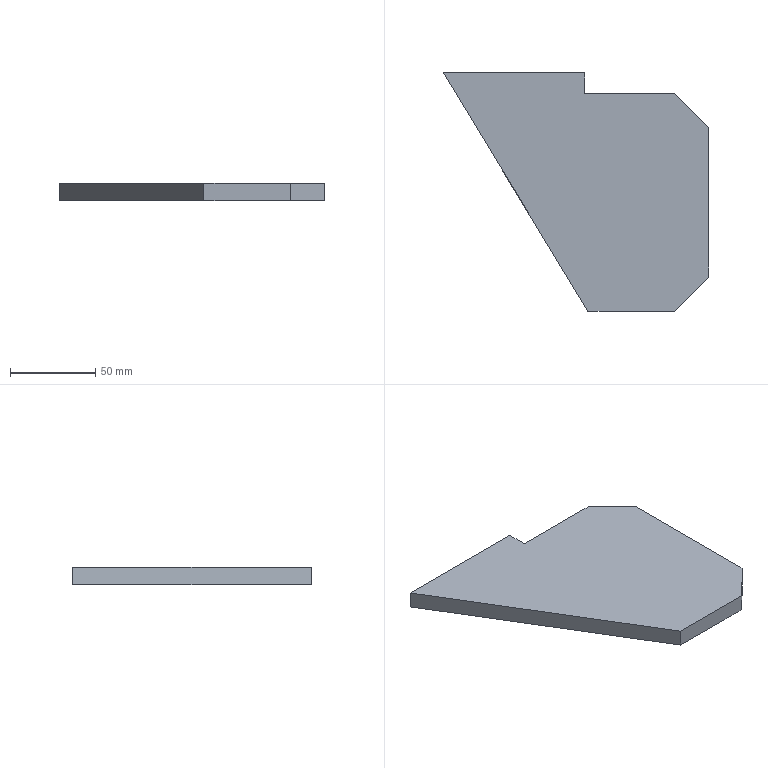Part | STEP file | 07 Rib plate | 1 solid | 10 faces | box 156 x 140 x 10 mm | volume 146140 mm3 | plane 10
STEP:
#1=CARTESIAN_POINT('',(0.,0.,0.));
#2=DIRECTION('',(0.,0.,1.));
#3=DIRECTION('',(1.,0.,0.));
#4=AXIS2_PLACEMENT_3D('',#1,#2,#3);
#5=CARTESIAN_POINT('',(0.,0.,0.));
#6=VERTEX_POINT('',#5);
#7=CARTESIAN_POINT('',(85.,-140.,0.));
#8=VERTEX_POINT('',#7);
#9=CARTESIAN_POINT('',(0.,0.,0.));
#10=DIRECTION('',(0.519,-0.8548,0.));
#11=VECTOR('',#10,1.);
#12=LINE('',#9,#11);
#13=CARTESIAN_POINT('',(0.,0.,10.));
#14=DIRECTION('',(0.8548,0.519,0.));
#15=DIRECTION('',(-0.519,0.8548,0.));
#16=AXIS2_PLACEMENT_3D('',#13,#14,#15);
#17=PLANE('',#16);
#18=CARTESIAN_POINT('',(0.,-10.));
#19=DIRECTION('',(-1.,0.));
#20=VECTOR('',#19,1.);
#21=LINE('',#18,#20);
#22=(GEOMETRIC_REPRESENTATION_CONTEXT(2)PARAMETRIC_REPRESENTATION_CONTEXT()REPRESENTATION_CONTEXT('',''));
#23=DEFINITIONAL_REPRESENTATION('',(#21),#22);
#24=PCURVE('',#17,#23);
#25=CARTESIAN_POINT('',(0.,0.,0.));
#26=DIRECTION('',(0.,0.,-1.));
#27=DIRECTION('',(-1.,0.,0.));
#28=AXIS2_PLACEMENT_3D('',#25,#26,#27);
#29=PLANE('',#28);
#30=CARTESIAN_POINT('',(0.,0.));
#31=DIRECTION('',(-0.519,-0.8548));
#32=VECTOR('',#31,1.);
#33=LINE('',#30,#32);
#34=(GEOMETRIC_REPRESENTATION_CONTEXT(2)PARAMETRIC_REPRESENTATION_CONTEXT()REPRESENTATION_CONTEXT('',''));
#35=DEFINITIONAL_REPRESENTATION('',(#33),#34);
#36=PCURVE('',#29,#35);
#37=SURFACE_CURVE('',#12,(#24,#36),.PCURVE_S1.);
#38=EDGE_CURVE('',#6,#8,#37,.T.);
#39=ORIENTED_EDGE('',*,*,#38,.T.);
#40=CARTESIAN_POINT('',(85.,-140.,10.));
#41=VERTEX_POINT('',#40);
#42=CARTESIAN_POINT('',(85.,-140.,10.));
#43=DIRECTION('',(0.,0.,-1.));
#44=VECTOR('',#43,1.);
#45=LINE('',#42,#44);
#46=CARTESIAN_POINT('',(-163.783,0.));
#47=DIRECTION('',(0.,-1.));
#48=VECTOR('',#47,1.);
#49=LINE('',#46,#48);
#50=(GEOMETRIC_REPRESENTATION_CONTEXT(2)PARAMETRIC_REPRESENTATION_CONTEXT()REPRESENTATION_CONTEXT('',''));
#51=DEFINITIONAL_REPRESENTATION('',(#49),#50);
#52=PCURVE('',#17,#51);
#53=CARTESIAN_POINT('',(85.,-140.,10.));
#54=DIRECTION('',(0.,1.,0.));
#55=DIRECTION('',(0.,0.,1.));
#56=AXIS2_PLACEMENT_3D('',#53,#54,#55);
#57=PLANE('',#56);
#58=CARTESIAN_POINT('',(0.,0.));
#59=DIRECTION('',(-1.,0.));
#60=VECTOR('',#59,1.);
#61=LINE('',#58,#60);
#62=(GEOMETRIC_REPRESENTATION_CONTEXT(2)PARAMETRIC_REPRESENTATION_CONTEXT()REPRESENTATION_CONTEXT('',''));
#63=DEFINITIONAL_REPRESENTATION('',(#61),#62);
#64=PCURVE('',#57,#63);
#65=SURFACE_CURVE('',#45,(#52,#64),.PCURVE_S1.);
#66=EDGE_CURVE('',#41,#8,#65,.T.);
#67=ORIENTED_EDGE('',*,*,#66,.F.);
#68=CARTESIAN_POINT('',(0.,0.,10.));
#69=VERTEX_POINT('',#68);
#70=CARTESIAN_POINT('',(0.,0.,10.));
#71=DIRECTION('',(0.519,-0.8548,0.));
#72=VECTOR('',#71,1.);
#73=LINE('',#70,#72);
#74=CARTESIAN_POINT('',(0.,0.));
#75=DIRECTION('',(-1.,0.));
#76=VECTOR('',#75,1.);
#77=LINE('',#74,#76);
#78=(GEOMETRIC_REPRESENTATION_CONTEXT(2)PARAMETRIC_REPRESENTATION_CONTEXT()REPRESENTATION_CONTEXT('',''));
#79=DEFINITIONAL_REPRESENTATION('',(#77),#78);
#80=PCURVE('',#17,#79);
#81=CARTESIAN_POINT('',(0.,0.,10.));
#82=DIRECTION('',(0.,0.,-1.));
#83=DIRECTION('',(-1.,0.,0.));
#84=AXIS2_PLACEMENT_3D('',#81,#82,#83);
#85=PLANE('',#84);
#86=CARTESIAN_POINT('',(0.,0.));
#87=DIRECTION('',(-0.519,-0.8548));
#88=VECTOR('',#87,1.);
#89=LINE('',#86,#88);
#90=(GEOMETRIC_REPRESENTATION_CONTEXT(2)PARAMETRIC_REPRESENTATION_CONTEXT()REPRESENTATION_CONTEXT('',''));
#91=DEFINITIONAL_REPRESENTATION('',(#89),#90);
#92=PCURVE('',#85,#91);
#93=SURFACE_CURVE('',#73,(#80,#92),.PCURVE_S1.);
#94=EDGE_CURVE('',#69,#41,#93,.T.);
#95=ORIENTED_EDGE('',*,*,#94,.F.);
#96=CARTESIAN_POINT('',(0.,0.,10.));
#97=DIRECTION('',(0.,0.,-1.));
#98=VECTOR('',#97,1.);
#99=LINE('',#96,#98);
#100=CARTESIAN_POINT('',(0.,0.));
#101=DIRECTION('',(0.,-1.));
#102=VECTOR('',#101,1.);
#103=LINE('',#100,#102);
#104=(GEOMETRIC_REPRESENTATION_CONTEXT(2)PARAMETRIC_REPRESENTATION_CONTEXT()REPRESENTATION_CONTEXT('',''));
#105=DEFINITIONAL_REPRESENTATION('',(#103),#104);
#106=PCURVE('',#17,#105);
#107=CARTESIAN_POINT('',(0.,0.,10.));
#108=DIRECTION('',(0.,-1.,0.));
#109=DIRECTION('',(0.,0.,-1.));
#110=AXIS2_PLACEMENT_3D('',#107,#108,#109);
#111=PLANE('',#110);
#112=CARTESIAN_POINT('',(0.,0.));
#113=DIRECTION('',(1.,0.));
#114=VECTOR('',#113,1.);
#115=LINE('',#112,#114);
#116=(GEOMETRIC_REPRESENTATION_CONTEXT(2)PARAMETRIC_REPRESENTATION_CONTEXT()REPRESENTATION_CONTEXT('',''));
#117=DEFINITIONAL_REPRESENTATION('',(#115),#116);
#118=PCURVE('',#111,#117);
#119=SURFACE_CURVE('',#99,(#106,#118),.PCURVE_S1.);
#120=EDGE_CURVE('',#69,#6,#119,.T.);
#121=ORIENTED_EDGE('',*,*,#120,.T.);
#122=EDGE_LOOP('',(#39,#67,#95,#121));
#123=FACE_BOUND('',#122,.T.);
#124=ADVANCED_FACE('',(#123),#17,.F.);
#125=CARTESIAN_POINT('',(136.,-140.,0.));
#126=VERTEX_POINT('',#125);
#127=CARTESIAN_POINT('',(85.,-140.,0.));
#128=DIRECTION('',(1.,0.,0.));
#129=VECTOR('',#128,1.);
#130=LINE('',#127,#129);
#131=CARTESIAN_POINT('',(-10.,0.));
#132=DIRECTION('',(0.,1.));
#133=VECTOR('',#132,1.);
#134=LINE('',#131,#133);
#135=(GEOMETRIC_REPRESENTATION_CONTEXT(2)PARAMETRIC_REPRESENTATION_CONTEXT()REPRESENTATION_CONTEXT('',''));
#136=DEFINITIONAL_REPRESENTATION('',(#134),#135);
#137=PCURVE('',#57,#136);
#138=CARTESIAN_POINT('',(-85.,-140.));
#139=DIRECTION('',(-1.,0.));
#140=VECTOR('',#139,1.);
#141=LINE('',#138,#140);
#142=(GEOMETRIC_REPRESENTATION_CONTEXT(2)PARAMETRIC_REPRESENTATION_CONTEXT()REPRESENTATION_CONTEXT('',''));
#143=DEFINITIONAL_REPRESENTATION('',(#141),#142);
#144=PCURVE('',#29,#143);
#145=SURFACE_CURVE('',#130,(#137,#144),.PCURVE_S1.);
#146=EDGE_CURVE('',#8,#126,#145,.T.);
#147=ORIENTED_EDGE('',*,*,#146,.T.);
#148=CARTESIAN_POINT('',(136.,-140.,10.));
#149=VERTEX_POINT('',#148);
#150=CARTESIAN_POINT('',(136.,-140.,10.));
#151=DIRECTION('',(0.,0.,-1.));
#152=VECTOR('',#151,1.);
#153=LINE('',#150,#152);
#154=CARTESIAN_POINT('',(0.,51.));
#155=DIRECTION('',(-1.,0.));
#156=VECTOR('',#155,1.);
#157=LINE('',#154,#156);
#158=(GEOMETRIC_REPRESENTATION_CONTEXT(2)PARAMETRIC_REPRESENTATION_CONTEXT()REPRESENTATION_CONTEXT('',''));
#159=DEFINITIONAL_REPRESENTATION('',(#157),#158);
#160=PCURVE('',#57,#159);
#161=CARTESIAN_POINT('',(156.,-120.,10.));
#162=DIRECTION('',(-0.7071,0.7071,0.));
#163=DIRECTION('',(-0.7071,-0.7071,0.));
#164=AXIS2_PLACEMENT_3D('',#161,#162,#163);
#165=PLANE('',#164);
#166=CARTESIAN_POINT('',(28.284,0.));
#167=DIRECTION('',(0.,-1.));
#168=VECTOR('',#167,1.);
#169=LINE('',#166,#168);
#170=(GEOMETRIC_REPRESENTATION_CONTEXT(2)PARAMETRIC_REPRESENTATION_CONTEXT()REPRESENTATION_CONTEXT('',''));
#171=DEFINITIONAL_REPRESENTATION('',(#169),#170);
#172=PCURVE('',#165,#171);
#173=SURFACE_CURVE('',#153,(#160,#172),.PCURVE_S1.);
#174=EDGE_CURVE('',#149,#126,#173,.T.);
#175=ORIENTED_EDGE('',*,*,#174,.F.);
#176=CARTESIAN_POINT('',(85.,-140.,10.));
#177=DIRECTION('',(1.,0.,0.));
#178=VECTOR('',#177,1.);
#179=LINE('',#176,#178);
#180=CARTESIAN_POINT('',(0.,0.));
#181=DIRECTION('',(0.,1.));
#182=VECTOR('',#181,1.);
#183=LINE('',#180,#182);
#184=(GEOMETRIC_REPRESENTATION_CONTEXT(2)PARAMETRIC_REPRESENTATION_CONTEXT()REPRESENTATION_CONTEXT('',''));
#185=DEFINITIONAL_REPRESENTATION('',(#183),#184);
#186=PCURVE('',#57,#185);
#187=CARTESIAN_POINT('',(-85.,-140.));
#188=DIRECTION('',(-1.,0.));
#189=VECTOR('',#188,1.);
#190=LINE('',#187,#189);
#191=(GEOMETRIC_REPRESENTATION_CONTEXT(2)PARAMETRIC_REPRESENTATION_CONTEXT()REPRESENTATION_CONTEXT('',''));
#192=DEFINITIONAL_REPRESENTATION('',(#190),#191);
#193=PCURVE('',#85,#192);
#194=SURFACE_CURVE('',#179,(#186,#193),.PCURVE_S1.);
#195=EDGE_CURVE('',#41,#149,#194,.T.);
#196=ORIENTED_EDGE('',*,*,#195,.F.);
#197=ORIENTED_EDGE('',*,*,#66,.T.);
#198=EDGE_LOOP('',(#147,#175,#196,#197));
#199=FACE_BOUND('',#198,.T.);
#200=ADVANCED_FACE('',(#199),#57,.F.);
#201=CARTESIAN_POINT('',(156.,-120.,0.));
#202=VERTEX_POINT('',#201);
#203=CARTESIAN_POINT('',(156.,-120.,0.));
#204=DIRECTION('',(0.7071,0.7071,0.));
#205=VECTOR('',#204,1.);
#206=LINE('',#203,#205);
#207=CARTESIAN_POINT('',(0.,-10.));
#208=DIRECTION('',(-1.,0.));
#209=VECTOR('',#208,1.);
#210=LINE('',#207,#209);
#211=(GEOMETRIC_REPRESENTATION_CONTEXT(2)PARAMETRIC_REPRESENTATION_CONTEXT()REPRESENTATION_CONTEXT('',''));
#212=DEFINITIONAL_REPRESENTATION('',(#210),#211);
#213=PCURVE('',#165,#212);
#214=CARTESIAN_POINT('',(-156.,-120.));
#215=DIRECTION('',(-0.7071,0.7071));
#216=VECTOR('',#215,1.);
#217=LINE('',#214,#216);
#218=(GEOMETRIC_REPRESENTATION_CONTEXT(2)PARAMETRIC_REPRESENTATION_CONTEXT()REPRESENTATION_CONTEXT('',''));
#219=DEFINITIONAL_REPRESENTATION('',(#217),#218);
#220=PCURVE('',#29,#219);
#221=SURFACE_CURVE('',#206,(#213,#220),.PCURVE_S1.);
#222=EDGE_CURVE('',#126,#202,#221,.T.);
#223=ORIENTED_EDGE('',*,*,#222,.T.);
#224=CARTESIAN_POINT('',(156.,-120.,10.));
#225=VERTEX_POINT('',#224);
#226=CARTESIAN_POINT('',(156.,-120.,10.));
#227=DIRECTION('',(0.,0.,-1.));
#228=VECTOR('',#227,1.);
#229=LINE('',#226,#228);
#230=CARTESIAN_POINT('',(0.,0.));
#231=DIRECTION('',(0.,-1.));
#232=VECTOR('',#231,1.);
#233=LINE('',#230,#232);
#234=(GEOMETRIC_REPRESENTATION_CONTEXT(2)PARAMETRIC_REPRESENTATION_CONTEXT()REPRESENTATION_CONTEXT('',''));
#235=DEFINITIONAL_REPRESENTATION('',(#233),#234);
#236=PCURVE('',#165,#235);
#237=CARTESIAN_POINT('',(156.,-32.,10.));
#238=DIRECTION('',(-1.,0.,0.));
#239=DIRECTION('',(0.,-1.,0.));
#240=AXIS2_PLACEMENT_3D('',#237,#238,#239);
#241=PLANE('',#240);
#242=CARTESIAN_POINT('',(88.,0.));
#243=DIRECTION('',(0.,-1.));
#244=VECTOR('',#243,1.);
#245=LINE('',#242,#244);
#246=(GEOMETRIC_REPRESENTATION_CONTEXT(2)PARAMETRIC_REPRESENTATION_CONTEXT()REPRESENTATION_CONTEXT('',''));
#247=DEFINITIONAL_REPRESENTATION('',(#245),#246);
#248=PCURVE('',#241,#247);
#249=SURFACE_CURVE('',#229,(#236,#248),.PCURVE_S1.);
#250=EDGE_CURVE('',#225,#202,#249,.T.);
#251=ORIENTED_EDGE('',*,*,#250,.F.);
#252=CARTESIAN_POINT('',(156.,-120.,10.));
#253=DIRECTION('',(0.7071,0.7071,0.));
#254=VECTOR('',#253,1.);
#255=LINE('',#252,#254);
#256=CARTESIAN_POINT('',(0.,0.));
#257=DIRECTION('',(-1.,0.));
#258=VECTOR('',#257,1.);
#259=LINE('',#256,#258);
#260=(GEOMETRIC_REPRESENTATION_CONTEXT(2)PARAMETRIC_REPRESENTATION_CONTEXT()REPRESENTATION_CONTEXT('',''));
#261=DEFINITIONAL_REPRESENTATION('',(#259),#260);
#262=PCURVE('',#165,#261);
#263=CARTESIAN_POINT('',(-156.,-120.));
#264=DIRECTION('',(-0.7071,0.7071));
#265=VECTOR('',#264,1.);
#266=LINE('',#263,#265);
#267=(GEOMETRIC_REPRESENTATION_CONTEXT(2)PARAMETRIC_REPRESENTATION_CONTEXT()REPRESENTATION_CONTEXT('',''));
#268=DEFINITIONAL_REPRESENTATION('',(#266),#267);
#269=PCURVE('',#85,#268);
#270=SURFACE_CURVE('',#255,(#262,#269),.PCURVE_S1.);
#271=EDGE_CURVE('',#149,#225,#270,.T.);
#272=ORIENTED_EDGE('',*,*,#271,.F.);
#273=ORIENTED_EDGE('',*,*,#174,.T.);
#274=EDGE_LOOP('',(#223,#251,#272,#273));
#275=FACE_BOUND('',#274,.T.);
#276=ADVANCED_FACE('',(#275),#165,.F.);
#277=CARTESIAN_POINT('',(156.,-32.,0.));
#278=VERTEX_POINT('',#277);
#279=CARTESIAN_POINT('',(156.,-32.,0.));
#280=DIRECTION('',(0.,1.,0.));
#281=VECTOR('',#280,1.);
#282=LINE('',#279,#281);
#283=CARTESIAN_POINT('',(0.,-10.));
#284=DIRECTION('',(-1.,0.));
#285=VECTOR('',#284,1.);
#286=LINE('',#283,#285);
#287=(GEOMETRIC_REPRESENTATION_CONTEXT(2)PARAMETRIC_REPRESENTATION_CONTEXT()REPRESENTATION_CONTEXT('',''));
#288=DEFINITIONAL_REPRESENTATION('',(#286),#287);
#289=PCURVE('',#241,#288);
#290=CARTESIAN_POINT('',(-156.,-32.));
#291=DIRECTION('',(0.,1.));
#292=VECTOR('',#291,1.);
#293=LINE('',#290,#292);
#294=(GEOMETRIC_REPRESENTATION_CONTEXT(2)PARAMETRIC_REPRESENTATION_CONTEXT()REPRESENTATION_CONTEXT('',''));
#295=DEFINITIONAL_REPRESENTATION('',(#293),#294);
#296=PCURVE('',#29,#295);
#297=SURFACE_CURVE('',#282,(#289,#296),.PCURVE_S1.);
#298=EDGE_CURVE('',#202,#278,#297,.T.);
#299=ORIENTED_EDGE('',*,*,#298,.T.);
#300=CARTESIAN_POINT('',(156.,-32.,10.));
#301=VERTEX_POINT('',#300);
#302=CARTESIAN_POINT('',(156.,-32.,10.));
#303=DIRECTION('',(0.,0.,-1.));
#304=VECTOR('',#303,1.);
#305=LINE('',#302,#304);
#306=CARTESIAN_POINT('',(0.,0.));
#307=DIRECTION('',(0.,-1.));
#308=VECTOR('',#307,1.);
#309=LINE('',#306,#308);
#310=(GEOMETRIC_REPRESENTATION_CONTEXT(2)PARAMETRIC_REPRESENTATION_CONTEXT()REPRESENTATION_CONTEXT('',''));
#311=DEFINITIONAL_REPRESENTATION('',(#309),#310);
#312=PCURVE('',#241,#311);
#313=CARTESIAN_POINT('',(136.,-12.,10.));
#314=DIRECTION('',(-0.7071,-0.7071,0.));
#315=DIRECTION('',(0.7071,-0.7071,0.));
#316=AXIS2_PLACEMENT_3D('',#313,#314,#315);
#317=PLANE('',#316);
#318=CARTESIAN_POINT('',(28.284,0.));
#319=DIRECTION('',(0.,-1.));
#320=VECTOR('',#319,1.);
#321=LINE('',#318,#320);
#322=(GEOMETRIC_REPRESENTATION_CONTEXT(2)PARAMETRIC_REPRESENTATION_CONTEXT()REPRESENTATION_CONTEXT('',''));
#323=DEFINITIONAL_REPRESENTATION('',(#321),#322);
#324=PCURVE('',#317,#323);
#325=SURFACE_CURVE('',#305,(#312,#324),.PCURVE_S1.);
#326=EDGE_CURVE('',#301,#278,#325,.T.);
#327=ORIENTED_EDGE('',*,*,#326,.F.);
#328=CARTESIAN_POINT('',(156.,-32.,10.));
#329=DIRECTION('',(0.,1.,0.));
#330=VECTOR('',#329,1.);
#331=LINE('',#328,#330);
#332=CARTESIAN_POINT('',(0.,0.));
#333=DIRECTION('',(-1.,0.));
#334=VECTOR('',#333,1.);
#335=LINE('',#332,#334);
#336=(GEOMETRIC_REPRESENTATION_CONTEXT(2)PARAMETRIC_REPRESENTATION_CONTEXT()REPRESENTATION_CONTEXT('',''));
#337=DEFINITIONAL_REPRESENTATION('',(#335),#336);
#338=PCURVE('',#241,#337);
#339=CARTESIAN_POINT('',(-156.,-32.));
#340=DIRECTION('',(0.,1.));
#341=VECTOR('',#340,1.);
#342=LINE('',#339,#341);
#343=(GEOMETRIC_REPRESENTATION_CONTEXT(2)PARAMETRIC_REPRESENTATION_CONTEXT()REPRESENTATION_CONTEXT('',''));
#344=DEFINITIONAL_REPRESENTATION('',(#342),#343);
#345=PCURVE('',#85,#344);
#346=SURFACE_CURVE('',#331,(#338,#345),.PCURVE_S1.);
#347=EDGE_CURVE('',#225,#301,#346,.T.);
#348=ORIENTED_EDGE('',*,*,#347,.F.);
#349=ORIENTED_EDGE('',*,*,#250,.T.);
#350=EDGE_LOOP('',(#299,#327,#348,#349));
#351=FACE_BOUND('',#350,.T.);
#352=ADVANCED_FACE('',(#351),#241,.F.);
#353=CARTESIAN_POINT('',(136.,-12.,0.));
#354=VERTEX_POINT('',#353);
#355=CARTESIAN_POINT('',(136.,-12.,0.));
#356=DIRECTION('',(-0.7071,0.7071,0.));
#357=VECTOR('',#356,1.);
#358=LINE('',#355,#357);
#359=CARTESIAN_POINT('',(0.,-10.));
#360=DIRECTION('',(-1.,0.));
#361=VECTOR('',#360,1.);
#362=LINE('',#359,#361);
#363=(GEOMETRIC_REPRESENTATION_CONTEXT(2)PARAMETRIC_REPRESENTATION_CONTEXT()REPRESENTATION_CONTEXT('',''));
#364=DEFINITIONAL_REPRESENTATION('',(#362),#363);
#365=PCURVE('',#317,#364);
#366=CARTESIAN_POINT('',(-136.,-12.));
#367=DIRECTION('',(0.7071,0.7071));
#368=VECTOR('',#367,1.);
#369=LINE('',#366,#368);
#370=(GEOMETRIC_REPRESENTATION_CONTEXT(2)PARAMETRIC_REPRESENTATION_CONTEXT()REPRESENTATION_CONTEXT('',''));
#371=DEFINITIONAL_REPRESENTATION('',(#369),#370);
#372=PCURVE('',#29,#371);
#373=SURFACE_CURVE('',#358,(#365,#372),.PCURVE_S1.);
#374=EDGE_CURVE('',#278,#354,#373,.T.);
#375=ORIENTED_EDGE('',*,*,#374,.T.);
#376=CARTESIAN_POINT('',(136.,-12.,10.));
#377=VERTEX_POINT('',#376);
#378=CARTESIAN_POINT('',(136.,-12.,10.));
#379=DIRECTION('',(0.,0.,-1.));
#380=VECTOR('',#379,1.);
#381=LINE('',#378,#380);
#382=CARTESIAN_POINT('',(0.,0.));
#383=DIRECTION('',(0.,-1.));
#384=VECTOR('',#383,1.);
#385=LINE('',#382,#384);
#386=(GEOMETRIC_REPRESENTATION_CONTEXT(2)PARAMETRIC_REPRESENTATION_CONTEXT()REPRESENTATION_CONTEXT('',''));
#387=DEFINITIONAL_REPRESENTATION('',(#385),#386);
#388=PCURVE('',#317,#387);
#389=CARTESIAN_POINT('',(83.,-12.,10.));
#390=DIRECTION('',(0.,-1.,0.));
#391=DIRECTION('',(1.,0.,0.));
#392=AXIS2_PLACEMENT_3D('',#389,#390,#391);
#393=PLANE('',#392);
#394=CARTESIAN_POINT('',(53.,0.));
#395=DIRECTION('',(0.,-1.));
#396=VECTOR('',#395,1.);
#397=LINE('',#394,#396);
#398=(GEOMETRIC_REPRESENTATION_CONTEXT(2)PARAMETRIC_REPRESENTATION_CONTEXT()REPRESENTATION_CONTEXT('',''));
#399=DEFINITIONAL_REPRESENTATION('',(#397),#398);
#400=PCURVE('',#393,#399);
#401=SURFACE_CURVE('',#381,(#388,#400),.PCURVE_S1.);
#402=EDGE_CURVE('',#377,#354,#401,.T.);
#403=ORIENTED_EDGE('',*,*,#402,.F.);
#404=CARTESIAN_POINT('',(136.,-12.,10.));
#405=DIRECTION('',(-0.7071,0.7071,0.));
#406=VECTOR('',#405,1.);
#407=LINE('',#404,#406);
#408=CARTESIAN_POINT('',(0.,0.));
#409=DIRECTION('',(-1.,0.));
#410=VECTOR('',#409,1.);
#411=LINE('',#408,#410);
#412=(GEOMETRIC_REPRESENTATION_CONTEXT(2)PARAMETRIC_REPRESENTATION_CONTEXT()REPRESENTATION_CONTEXT('',''));
#413=DEFINITIONAL_REPRESENTATION('',(#411),#412);
#414=PCURVE('',#317,#413);
#415=CARTESIAN_POINT('',(-136.,-12.));
#416=DIRECTION('',(0.7071,0.7071));
#417=VECTOR('',#416,1.);
#418=LINE('',#415,#417);
#419=(GEOMETRIC_REPRESENTATION_CONTEXT(2)PARAMETRIC_REPRESENTATION_CONTEXT()REPRESENTATION_CONTEXT('',''));
#420=DEFINITIONAL_REPRESENTATION('',(#418),#419);
#421=PCURVE('',#85,#420);
#422=SURFACE_CURVE('',#407,(#414,#421),.PCURVE_S1.);
#423=EDGE_CURVE('',#301,#377,#422,.T.);
#424=ORIENTED_EDGE('',*,*,#423,.F.);
#425=ORIENTED_EDGE('',*,*,#326,.T.);
#426=EDGE_LOOP('',(#375,#403,#424,#425));
#427=FACE_BOUND('',#426,.T.);
#428=ADVANCED_FACE('',(#427),#317,.F.);
#429=CARTESIAN_POINT('',(83.,-12.,0.));
#430=VERTEX_POINT('',#429);
#431=CARTESIAN_POINT('',(83.,-12.,0.));
#432=DIRECTION('',(-1.,0.,0.));
#433=VECTOR('',#432,1.);
#434=LINE('',#431,#433);
#435=CARTESIAN_POINT('',(0.,-10.));
#436=DIRECTION('',(-1.,0.));
#437=VECTOR('',#436,1.);
#438=LINE('',#435,#437);
#439=(GEOMETRIC_REPRESENTATION_CONTEXT(2)PARAMETRIC_REPRESENTATION_CONTEXT()REPRESENTATION_CONTEXT('',''));
#440=DEFINITIONAL_REPRESENTATION('',(#438),#439);
#441=PCURVE('',#393,#440);
#442=CARTESIAN_POINT('',(-83.,-12.));
#443=DIRECTION('',(1.,0.));
#444=VECTOR('',#443,1.);
#445=LINE('',#442,#444);
#446=(GEOMETRIC_REPRESENTATION_CONTEXT(2)PARAMETRIC_REPRESENTATION_CONTEXT()REPRESENTATION_CONTEXT('',''));
#447=DEFINITIONAL_REPRESENTATION('',(#445),#446);
#448=PCURVE('',#29,#447);
#449=SURFACE_CURVE('',#434,(#441,#448),.PCURVE_S1.);
#450=EDGE_CURVE('',#354,#430,#449,.T.);
#451=ORIENTED_EDGE('',*,*,#450,.T.);
#452=CARTESIAN_POINT('',(83.,-12.,10.));
#453=VERTEX_POINT('',#452);
#454=CARTESIAN_POINT('',(83.,-12.,10.));
#455=DIRECTION('',(0.,0.,-1.));
#456=VECTOR('',#455,1.);
#457=LINE('',#454,#456);
#458=CARTESIAN_POINT('',(0.,0.));
#459=DIRECTION('',(0.,-1.));
#460=VECTOR('',#459,1.);
#461=LINE('',#458,#460);
#462=(GEOMETRIC_REPRESENTATION_CONTEXT(2)PARAMETRIC_REPRESENTATION_CONTEXT()REPRESENTATION_CONTEXT('',''));
#463=DEFINITIONAL_REPRESENTATION('',(#461),#462);
#464=PCURVE('',#393,#463);
#465=CARTESIAN_POINT('',(83.,0.,10.));
#466=DIRECTION('',(-1.,0.,0.));
#467=DIRECTION('',(0.,0.,1.));
#468=AXIS2_PLACEMENT_3D('',#465,#466,#467);
#469=PLANE('',#468);
#470=CARTESIAN_POINT('',(0.,-12.));
#471=DIRECTION('',(-1.,0.));
#472=VECTOR('',#471,1.);
#473=LINE('',#470,#472);
#474=(GEOMETRIC_REPRESENTATION_CONTEXT(2)PARAMETRIC_REPRESENTATION_CONTEXT()REPRESENTATION_CONTEXT('',''));
#475=DEFINITIONAL_REPRESENTATION('',(#473),#474);
#476=PCURVE('',#469,#475);
#477=SURFACE_CURVE('',#457,(#464,#476),.PCURVE_S1.);
#478=EDGE_CURVE('',#453,#430,#477,.T.);
#479=ORIENTED_EDGE('',*,*,#478,.F.);
#480=CARTESIAN_POINT('',(83.,-12.,10.));
#481=DIRECTION('',(-1.,0.,0.));
#482=VECTOR('',#481,1.);
#483=LINE('',#480,#482);
#484=CARTESIAN_POINT('',(0.,0.));
#485=DIRECTION('',(-1.,0.));
#486=VECTOR('',#485,1.);
#487=LINE('',#484,#486);
#488=(GEOMETRIC_REPRESENTATION_CONTEXT(2)PARAMETRIC_REPRESENTATION_CONTEXT()REPRESENTATION_CONTEXT('',''));
#489=DEFINITIONAL_REPRESENTATION('',(#487),#488);
#490=PCURVE('',#393,#489);
#491=CARTESIAN_POINT('',(-83.,-12.));
#492=DIRECTION('',(1.,0.));
#493=VECTOR('',#492,1.);
#494=LINE('',#491,#493);
#495=(GEOMETRIC_REPRESENTATION_CONTEXT(2)PARAMETRIC_REPRESENTATION_CONTEXT()REPRESENTATION_CONTEXT('',''));
#496=DEFINITIONAL_REPRESENTATION('',(#494),#495);
#497=PCURVE('',#85,#496);
#498=SURFACE_CURVE('',#483,(#490,#497),.PCURVE_S1.);
#499=EDGE_CURVE('',#377,#453,#498,.T.);
#500=ORIENTED_EDGE('',*,*,#499,.F.);
#501=ORIENTED_EDGE('',*,*,#402,.T.);
#502=EDGE_LOOP('',(#451,#479,#500,#501));
#503=FACE_BOUND('',#502,.T.);
#504=ADVANCED_FACE('',(#503),#393,.F.);
#505=CARTESIAN_POINT('',(83.,0.,0.));
#506=VERTEX_POINT('',#505);
#507=CARTESIAN_POINT('',(83.,0.,0.));
#508=DIRECTION('',(0.,1.,0.));
#509=VECTOR('',#508,1.);
#510=LINE('',#507,#509);
#511=CARTESIAN_POINT('',(-10.,0.));
#512=DIRECTION('',(0.,1.));
#513=VECTOR('',#512,1.);
#514=LINE('',#511,#513);
#515=(GEOMETRIC_REPRESENTATION_CONTEXT(2)PARAMETRIC_REPRESENTATION_CONTEXT()REPRESENTATION_CONTEXT('',''));
#516=DEFINITIONAL_REPRESENTATION('',(#514),#515);
#517=PCURVE('',#469,#516);
#518=CARTESIAN_POINT('',(-83.,0.));
#519=DIRECTION('',(0.,1.));
#520=VECTOR('',#519,1.);
#521=LINE('',#518,#520);
#522=(GEOMETRIC_REPRESENTATION_CONTEXT(2)PARAMETRIC_REPRESENTATION_CONTEXT()REPRESENTATION_CONTEXT('',''));
#523=DEFINITIONAL_REPRESENTATION('',(#521),#522);
#524=PCURVE('',#29,#523);
#525=SURFACE_CURVE('',#510,(#517,#524),.PCURVE_S1.);
#526=EDGE_CURVE('',#430,#506,#525,.T.);
#527=ORIENTED_EDGE('',*,*,#526,.T.);
#528=CARTESIAN_POINT('',(83.,0.,10.));
#529=VERTEX_POINT('',#528);
#530=CARTESIAN_POINT('',(83.,0.,10.));
#531=DIRECTION('',(0.,0.,-1.));
#532=VECTOR('',#531,1.);
#533=LINE('',#530,#532);
#534=CARTESIAN_POINT('',(0.,0.));
#535=DIRECTION('',(-1.,0.));
#536=VECTOR('',#535,1.);
#537=LINE('',#534,#536);
#538=(GEOMETRIC_REPRESENTATION_CONTEXT(2)PARAMETRIC_REPRESENTATION_CONTEXT()REPRESENTATION_CONTEXT('',''));
#539=DEFINITIONAL_REPRESENTATION('',(#537),#538);
#540=PCURVE('',#469,#539);
#541=CARTESIAN_POINT('',(0.,83.));
#542=DIRECTION('',(1.,0.));
#543=VECTOR('',#542,1.);
#544=LINE('',#541,#543);
#545=(GEOMETRIC_REPRESENTATION_CONTEXT(2)PARAMETRIC_REPRESENTATION_CONTEXT()REPRESENTATION_CONTEXT('',''));
#546=DEFINITIONAL_REPRESENTATION('',(#544),#545);
#547=PCURVE('',#111,#546);
#548=SURFACE_CURVE('',#533,(#540,#547),.PCURVE_S1.);
#549=EDGE_CURVE('',#529,#506,#548,.T.);
#550=ORIENTED_EDGE('',*,*,#549,.F.);
#551=CARTESIAN_POINT('',(83.,0.,10.));
#552=DIRECTION('',(0.,1.,0.));
#553=VECTOR('',#552,1.);
#554=LINE('',#551,#553);
#555=CARTESIAN_POINT('',(0.,0.));
#556=DIRECTION('',(0.,1.));
#557=VECTOR('',#556,1.);
#558=LINE('',#555,#557);
#559=(GEOMETRIC_REPRESENTATION_CONTEXT(2)PARAMETRIC_REPRESENTATION_CONTEXT()REPRESENTATION_CONTEXT('',''));
#560=DEFINITIONAL_REPRESENTATION('',(#558),#559);
#561=PCURVE('',#469,#560);
#562=CARTESIAN_POINT('',(-83.,0.));
#563=DIRECTION('',(0.,1.));
#564=VECTOR('',#563,1.);
#565=LINE('',#562,#564);
#566=(GEOMETRIC_REPRESENTATION_CONTEXT(2)PARAMETRIC_REPRESENTATION_CONTEXT()REPRESENTATION_CONTEXT('',''));
#567=DEFINITIONAL_REPRESENTATION('',(#565),#566);
#568=PCURVE('',#85,#567);
#569=SURFACE_CURVE('',#554,(#561,#568),.PCURVE_S1.);
#570=EDGE_CURVE('',#453,#529,#569,.T.);
#571=ORIENTED_EDGE('',*,*,#570,.F.);
#572=ORIENTED_EDGE('',*,*,#478,.T.);
#573=EDGE_LOOP('',(#527,#550,#571,#572));
#574=FACE_BOUND('',#573,.T.);
#575=ADVANCED_FACE('',(#574),#469,.F.);
#576=CARTESIAN_POINT('',(0.,0.,0.));
#577=DIRECTION('',(-1.,0.,0.));
#578=VECTOR('',#577,1.);
#579=LINE('',#576,#578);
#580=CARTESIAN_POINT('',(10.,0.));
#581=DIRECTION('',(0.,-1.));
#582=VECTOR('',#581,1.);
#583=LINE('',#580,#582);
#584=(GEOMETRIC_REPRESENTATION_CONTEXT(2)PARAMETRIC_REPRESENTATION_CONTEXT()REPRESENTATION_CONTEXT('',''));
#585=DEFINITIONAL_REPRESENTATION('',(#583),#584);
#586=PCURVE('',#111,#585);
#587=CARTESIAN_POINT('',(0.,0.));
#588=DIRECTION('',(1.,0.));
#589=VECTOR('',#588,1.);
#590=LINE('',#587,#589);
#591=(GEOMETRIC_REPRESENTATION_CONTEXT(2)PARAMETRIC_REPRESENTATION_CONTEXT()REPRESENTATION_CONTEXT('',''));
#592=DEFINITIONAL_REPRESENTATION('',(#590),#591);
#593=PCURVE('',#29,#592);
#594=SURFACE_CURVE('',#579,(#586,#593),.PCURVE_S1.);
#595=EDGE_CURVE('',#506,#6,#594,.T.);
#596=ORIENTED_EDGE('',*,*,#595,.T.);
#597=ORIENTED_EDGE('',*,*,#120,.F.);
#598=CARTESIAN_POINT('',(0.,0.,10.));
#599=DIRECTION('',(-1.,0.,0.));
#600=VECTOR('',#599,1.);
#601=LINE('',#598,#600);
#602=CARTESIAN_POINT('',(0.,0.));
#603=DIRECTION('',(0.,-1.));
#604=VECTOR('',#603,1.);
#605=LINE('',#602,#604);
#606=(GEOMETRIC_REPRESENTATION_CONTEXT(2)PARAMETRIC_REPRESENTATION_CONTEXT()REPRESENTATION_CONTEXT('',''));
#607=DEFINITIONAL_REPRESENTATION('',(#605),#606);
#608=PCURVE('',#111,#607);
#609=CARTESIAN_POINT('',(0.,0.));
#610=DIRECTION('',(1.,0.));
#611=VECTOR('',#610,1.);
#612=LINE('',#609,#611);
#613=(GEOMETRIC_REPRESENTATION_CONTEXT(2)PARAMETRIC_REPRESENTATION_CONTEXT()REPRESENTATION_CONTEXT('',''));
#614=DEFINITIONAL_REPRESENTATION('',(#612),#613);
#615=PCURVE('',#85,#614);
#616=SURFACE_CURVE('',#601,(#608,#615),.PCURVE_S1.);
#617=EDGE_CURVE('',#529,#69,#616,.T.);
#618=ORIENTED_EDGE('',*,*,#617,.F.);
#619=ORIENTED_EDGE('',*,*,#549,.T.);
#620=EDGE_LOOP('',(#596,#597,#618,#619));
#621=FACE_BOUND('',#620,.T.);
#622=ADVANCED_FACE('',(#621),#111,.F.);
#623=ORIENTED_EDGE('',*,*,#94,.T.);
#624=ORIENTED_EDGE('',*,*,#195,.T.);
#625=ORIENTED_EDGE('',*,*,#271,.T.);
#626=ORIENTED_EDGE('',*,*,#347,.T.);
#627=ORIENTED_EDGE('',*,*,#423,.T.);
#628=ORIENTED_EDGE('',*,*,#499,.T.);
#629=ORIENTED_EDGE('',*,*,#570,.T.);
#630=ORIENTED_EDGE('',*,*,#617,.T.);
#631=EDGE_LOOP('',(#623,#624,#625,#626,#627,#628,#629,#630));
#632=FACE_BOUND('',#631,.T.);
#633=ADVANCED_FACE('',(#632),#85,.F.);
#634=ORIENTED_EDGE('',*,*,#38,.F.);
#635=ORIENTED_EDGE('',*,*,#595,.F.);
#636=ORIENTED_EDGE('',*,*,#526,.F.);
#637=ORIENTED_EDGE('',*,*,#450,.F.);
#638=ORIENTED_EDGE('',*,*,#374,.F.);
#639=ORIENTED_EDGE('',*,*,#298,.F.);
#640=ORIENTED_EDGE('',*,*,#222,.F.);
#641=ORIENTED_EDGE('',*,*,#146,.F.);
#642=EDGE_LOOP('',(#634,#635,#636,#637,#638,#639,#640,#641));
#643=FACE_BOUND('',#642,.T.);
#644=ADVANCED_FACE('',(#643),#29,.T.);
#645=CLOSED_SHELL('',(#124,#200,#276,#352,#428,#504,#575,#622,#633,#644));
#646=MANIFOLD_SOLID_BREP('',#645);
#647=(LENGTH_UNIT()NAMED_UNIT(*)SI_UNIT(.MILLI.,.METRE.));
#648=UNCERTAINTY_MEASURE_WITH_UNIT(LENGTH_MEASURE(0.0000001),#647,'','');
#649=(NAMED_UNIT(*)PLANE_ANGLE_UNIT()SI_UNIT($,.RADIAN.));
#650=(NAMED_UNIT(*)SI_UNIT($,.STERADIAN.)SOLID_ANGLE_UNIT());
#651=(GEOMETRIC_REPRESENTATION_CONTEXT(3)GLOBAL_UNCERTAINTY_ASSIGNED_CONTEXT((#648))GLOBAL_UNIT_ASSIGNED_CONTEXT((#647,#649,#650))REPRESENTATION_CONTEXT('',''));
#652=ADVANCED_BREP_SHAPE_REPRESENTATION('',(#4,#646),#651);